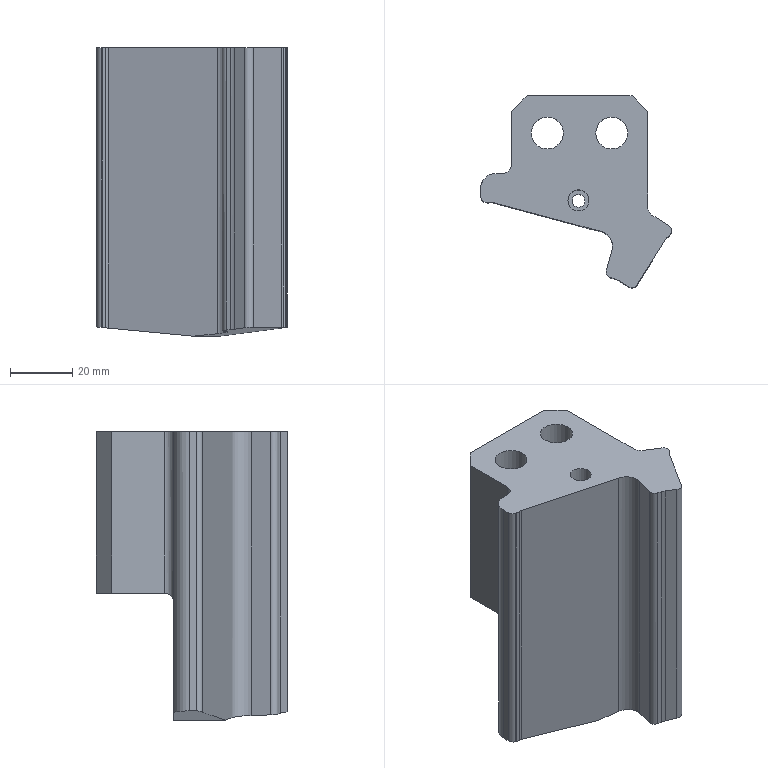Part | NX | features solid 2 | 1 solid | 46 faces | box 61.522 x 61.799 x 92.982 mm | volume 130232 mm3 | plane 22 | cylinder 22 | spline 1 | torus 1 | commonest cylinder face diameters 4 x8 6 x4 10 x4 10.3 x2 17 x2 4.1 x1
STEP:
#1=CARTESIAN_POINT('',(463.121,6.5,50.982));
#2=VERTEX_POINT('',#1);
#3=CARTESIAN_POINT('',(457.971,6.5,50.982));
#4=DIRECTION('',(-0.000000738,0.,-1.));
#5=DIRECTION('',(1.,0.,-0.000000738));
#6=AXIS2_PLACEMENT_3D('',#3,#4,#5);
#7=CIRCLE('',#6,5.15);
#8=EDGE_CURVE('',#2,#2,#7,.F.);
#9=ORIENTED_EDGE('',*,*,#8,.T.);
#10=EDGE_LOOP('',(#9));
#11=FACE_BOUND('',#10,.T.);
#12=CARTESIAN_POINT('',(449.471,6.5,50.982));
#13=VERTEX_POINT('',#12);
#14=CARTESIAN_POINT('',(457.971,6.5,50.982));
#15=DIRECTION('',(0.000000738,0.,1.));
#16=DIRECTION('',(-1.,0.,0.000000738));
#17=AXIS2_PLACEMENT_3D('',#14,#15,#16);
#18=CIRCLE('',#17,8.5);
#19=EDGE_CURVE('',#13,#13,#18,.T.);
#20=ORIENTED_EDGE('',*,*,#19,.F.);
#21=EDGE_LOOP('',(#20));
#22=FACE_BOUND('',#21,.T.);
#23=CARTESIAN_POINT('',(527.356,2.,50.982));
#24=DIRECTION('',(0.000000738,0.,1.));
#25=DIRECTION('',(1.,0.,-0.000000738));
#26=AXIS2_PLACEMENT_3D('',#23,#24,#25);
#27=PLANE('',#26);
#28=ADVANCED_FACE('',(#11,#22),#27,.F.);
#29=ORIENTED_EDGE('',*,*,#19,.T.);
#30=EDGE_LOOP('',(#29));
#31=FACE_BOUND('',#30,.T.);
#32=CARTESIAN_POINT('',(466.471,6.5,26.));
#33=VERTEX_POINT('',#32);
#34=CARTESIAN_POINT('',(457.971,6.5,26.));
#35=DIRECTION('',(0.,0.,1.));
#36=DIRECTION('',(1.,0.,0.));
#37=AXIS2_PLACEMENT_3D('',#34,#35,#36);
#38=CIRCLE('',#37,8.5);
#39=EDGE_CURVE('',#33,#33,#38,.F.);
#40=ORIENTED_EDGE('',*,*,#39,.T.);
#41=EDGE_LOOP('',(#40));
#42=FACE_BOUND('',#41,.T.);
#43=CARTESIAN_POINT('',(457.971,6.5,21.982));
#44=DIRECTION('',(0.000000369,-0.000000231,1.));
#45=DIRECTION('',(-1.,0.,0.000000369));
#46=AXIS2_PLACEMENT_3D('',#43,#44,#45);
#47=CYLINDRICAL_SURFACE('',#46,8.5);
#48=ADVANCED_FACE('',(#31,#42),#47,.F.);
#49=ORIENTED_EDGE('',*,*,#8,.F.);
#50=EDGE_LOOP('',(#49));
#51=FACE_BOUND('',#50,.T.);
#52=CARTESIAN_POINT('',(452.821,6.5,78.));
#53=VERTEX_POINT('',#52);
#54=CARTESIAN_POINT('',(457.971,6.5,78.));
#55=DIRECTION('',(0.,0.,-1.));
#56=DIRECTION('',(-1.,0.,0.));
#57=AXIS2_PLACEMENT_3D('',#54,#55,#56);
#58=CIRCLE('',#57,5.15);
#59=EDGE_CURVE('',#53,#53,#58,.F.);
#60=ORIENTED_EDGE('',*,*,#59,.T.);
#61=EDGE_LOOP('',(#60));
#62=FACE_BOUND('',#61,.T.);
#63=CARTESIAN_POINT('',(457.971,6.5,56.982));
#64=DIRECTION('',(0.000000369,-0.000000231,1.));
#65=DIRECTION('',(-1.,0.,0.000000369));
#66=AXIS2_PLACEMENT_3D('',#63,#64,#65);
#67=CYLINDRICAL_SURFACE('',#66,5.15);
#68=ADVANCED_FACE('',(#51,#62),#67,.F.);
#69=CARTESIAN_POINT('',(447.499,-13.166,-14.982));
#70=VERTEX_POINT('',#69);
#71=CARTESIAN_POINT('',(447.499,-17.238,-14.982));
#72=VERTEX_POINT('',#71);
#73=CARTESIAN_POINT('',(447.26,-15.202,-14.982));
#74=DIRECTION('',(-0.000000369,0.000000231,-1.));
#75=DIRECTION('',(-1.,0.,0.000000369));
#76=AXIS2_PLACEMENT_3D('',#73,#74,#75);
#77=CIRCLE('',#76,2.05);
#78=EDGE_CURVE('',#70,#72,#77,.T.);
#79=ORIENTED_EDGE('',*,*,#78,.F.);
#80=CARTESIAN_POINT('',(447.499,-6.5,-14.982));
#81=VERTEX_POINT('',#80);
#82=CARTESIAN_POINT('',(447.499,-13.942,-14.982));
#83=DIRECTION('',(0.,-1.,-0.000000231));
#84=VECTOR('',#83,1000.);
#85=LINE('',#82,#84);
#86=EDGE_CURVE('',#81,#70,#85,.T.);
#87=ORIENTED_EDGE('',*,*,#86,.F.);
#88=CARTESIAN_POINT('',(448.074,-6.5,-14.982));
#89=VERTEX_POINT('',#88);
#90=CARTESIAN_POINT('',(396.,-6.5,-14.982));
#91=DIRECTION('',(1.,0.,-0.000000369));
#92=VECTOR('',#91,1000.);
#93=LINE('',#90,#92);
#94=EDGE_CURVE('',#81,#89,#93,.T.);
#95=ORIENTED_EDGE('',*,*,#94,.T.);
#96=CARTESIAN_POINT('',(450.724,-7.26,-14.982));
#97=VERTEX_POINT('',#96);
#98=CARTESIAN_POINT('',(448.074,-11.5,-14.982));
#99=DIRECTION('',(0.000000369,-0.000000231,1.));
#100=DIRECTION('',(-1.,0.,0.000000369));
#101=AXIS2_PLACEMENT_3D('',#98,#99,#100);
#102=CIRCLE('',#101,5.);
#103=EDGE_CURVE('',#97,#89,#102,.T.);
#104=ORIENTED_EDGE('',*,*,#103,.F.);
#105=CARTESIAN_POINT('',(454.956,-9.904,-14.982));
#106=VERTEX_POINT('',#105);
#107=CARTESIAN_POINT('',(446.525,-4.636,-14.982));
#108=DIRECTION('',(0.848,-0.5299,-0.000000435));
#109=VECTOR('',#108,1000.);
#110=LINE('',#107,#109);
#111=EDGE_CURVE('',#97,#106,#110,.T.);
#112=ORIENTED_EDGE('',*,*,#111,.T.);
#113=CARTESIAN_POINT('',(447.499,-21.837,-14.982));
#114=VERTEX_POINT('',#113);
#115=CARTESIAN_POINT('',(452.665,-13.57,-14.982));
#116=DIRECTION('',(0.5299,0.848,0.));
#117=VECTOR('',#116,1000.);
#118=LINE('',#115,#117);
#119=EDGE_CURVE('',#114,#106,#118,.T.);
#120=ORIENTED_EDGE('',*,*,#119,.F.);
#121=CARTESIAN_POINT('',(447.499,-13.942,-14.982));
#122=DIRECTION('',(0.,-1.,-0.000000231));
#123=VECTOR('',#122,1000.);
#124=LINE('',#121,#123);
#125=EDGE_CURVE('',#72,#114,#124,.T.);
#126=ORIENTED_EDGE('',*,*,#125,.F.);
#127=EDGE_LOOP('',(#79,#87,#95,#104,#112,#120,#126));
#128=FACE_BOUND('',#127,.T.);
#129=CARTESIAN_POINT('',(393.129,-90.087,-14.982));
#130=DIRECTION('',(-0.000000369,0.000000231,-1.));
#131=DIRECTION('',(-1.,0.,0.000000369));
#132=AXIS2_PLACEMENT_3D('',#129,#130,#131);
#133=PLANE('',#132);
#134=ADVANCED_FACE('',(#128),#133,.T.);
#135=CARTESIAN_POINT('',(442.413,6.5,50.982));
#136=VERTEX_POINT('',#135);
#137=CARTESIAN_POINT('',(437.263,6.5,50.982));
#138=DIRECTION('',(0.,0.,-1.));
#139=DIRECTION('',(1.,0.,0.));
#140=AXIS2_PLACEMENT_3D('',#137,#138,#139);
#141=CIRCLE('',#140,5.15);
#142=EDGE_CURVE('',#136,#136,#141,.F.);
#143=ORIENTED_EDGE('',*,*,#142,.T.);
#144=EDGE_LOOP('',(#143));
#145=FACE_BOUND('',#144,.T.);
#146=CARTESIAN_POINT('',(445.763,6.5,50.982));
#147=VERTEX_POINT('',#146);
#148=CARTESIAN_POINT('',(437.263,6.5,50.982));
#149=DIRECTION('',(0.,0.,-1.));
#150=DIRECTION('',(1.,0.,0.));
#151=AXIS2_PLACEMENT_3D('',#148,#149,#150);
#152=CIRCLE('',#151,8.5);
#153=EDGE_CURVE('',#147,#147,#152,.F.);
#154=ORIENTED_EDGE('',*,*,#153,.F.);
#155=EDGE_LOOP('',(#154));
#156=FACE_BOUND('',#155,.T.);
#157=CARTESIAN_POINT('',(367.879,2.,50.982));
#158=DIRECTION('',(0.,0.,1.));
#159=DIRECTION('',(-1.,0.,0.));
#160=AXIS2_PLACEMENT_3D('',#157,#158,#159);
#161=PLANE('',#160);
#162=ADVANCED_FACE('',(#145,#156),#161,.F.);
#163=CARTESIAN_POINT('',(415.719,-11.5,-11.955));
#164=VERTEX_POINT('',#163);
#165=CARTESIAN_POINT('',(415.719,-11.5,78.));
#166=VERTEX_POINT('',#165);
#167=CARTESIAN_POINT('',(415.719,-11.5,-5.018));
#168=DIRECTION('',(0.000000369,-0.000000231,1.));
#169=VECTOR('',#168,1000.);
#170=LINE('',#167,#169);
#171=EDGE_CURVE('',#164,#166,#170,.T.);
#172=ORIENTED_EDGE('',*,*,#171,.T.);
#173=CARTESIAN_POINT('',(420.719,-6.5,78.));
#174=VERTEX_POINT('',#173);
#175=CARTESIAN_POINT('',(420.719,-11.5,78.));
#176=DIRECTION('',(0.,0.,-1.));
#177=DIRECTION('',(-1.,0.,0.));
#178=AXIS2_PLACEMENT_3D('',#175,#176,#177);
#179=CIRCLE('',#178,5.);
#180=EDGE_CURVE('',#174,#166,#179,.F.);
#181=ORIENTED_EDGE('',*,*,#180,.F.);
#182=CARTESIAN_POINT('',(420.719,-6.5,-12.431));
#183=VERTEX_POINT('',#182);
#184=CARTESIAN_POINT('',(420.719,-6.5,-5.018));
#185=DIRECTION('',(0.000000369,-0.000000231,1.));
#186=VECTOR('',#185,1000.);
#187=LINE('',#184,#186);
#188=EDGE_CURVE('',#183,#174,#187,.T.);
#189=ORIENTED_EDGE('',*,*,#188,.F.);
#190=CARTESIAN_POINT('',(420.719,-11.5,-12.431));
#191=DIRECTION('',(0.09481,-0.00000023,0.9955));
#192=DIRECTION('',(-0.9955,-0.000000022,0.09481));
#193=AXIS2_PLACEMENT_3D('',#190,#191,#192);
#194=ELLIPSE('',#193,5.023,5.);
#195=EDGE_CURVE('',#164,#183,#194,.F.);
#196=ORIENTED_EDGE('',*,*,#195,.F.);
#197=EDGE_LOOP('',(#172,#181,#189,#196));
#198=FACE_BOUND('',#197,.T.);
#199=CARTESIAN_POINT('',(420.719,-11.5,-5.018));
#200=DIRECTION('',(0.000000369,-0.000000231,1.));
#201=DIRECTION('',(1.,0.,-0.000000369));
#202=AXIS2_PLACEMENT_3D('',#199,#200,#201);
#203=CYLINDRICAL_SURFACE('',#202,5.);
#204=ADVANCED_FACE('',(#198),#203,.T.);
#205=CARTESIAN_POINT('',(415.719,-13.767,-11.955));
#206=VERTEX_POINT('',#205);
#207=CARTESIAN_POINT('',(415.719,-13.767,78.));
#208=VERTEX_POINT('',#207);
#209=CARTESIAN_POINT('',(415.719,-13.767,-5.018));
#210=DIRECTION('',(0.000000369,-0.000000231,1.));
#211=VECTOR('',#210,1000.);
#212=LINE('',#209,#211);
#213=EDGE_CURVE('',#206,#208,#212,.T.);
#214=ORIENTED_EDGE('',*,*,#213,.T.);
#215=CARTESIAN_POINT('',(415.719,-0.000000688,78.));
#216=DIRECTION('',(0.,-1.,0.));
#217=VECTOR('',#216,1000.);
#218=LINE('',#215,#217);
#219=EDGE_CURVE('',#166,#208,#218,.T.);
#220=ORIENTED_EDGE('',*,*,#219,.F.);
#221=ORIENTED_EDGE('',*,*,#171,.F.);
#222=CARTESIAN_POINT('',(415.719,-90.087,-11.955));
#223=DIRECTION('',(0.,1.,0.000000231));
#224=VECTOR('',#223,1000.);
#225=LINE('',#222,#224);
#226=EDGE_CURVE('',#206,#164,#225,.T.);
#227=ORIENTED_EDGE('',*,*,#226,.F.);
#228=EDGE_LOOP('',(#214,#220,#221,#227));
#229=FACE_BOUND('',#228,.T.);
#230=CARTESIAN_POINT('',(415.719,-89.912,-5.018));
#231=DIRECTION('',(1.,0.,-0.000000369));
#232=DIRECTION('',(-0.000000369,0.,-1.));
#233=AXIS2_PLACEMENT_3D('',#230,#231,#232);
#234=PLANE('',#233);
#235=ADVANCED_FACE('',(#229),#234,.F.);
#236=CARTESIAN_POINT('',(417.201,-15.698,-12.096));
#237=VERTEX_POINT('',#236);
#238=CARTESIAN_POINT('',(417.201,-15.698,78.));
#239=VERTEX_POINT('',#238);
#240=CARTESIAN_POINT('',(417.201,-15.698,-5.018));
#241=DIRECTION('',(0.000000369,-0.000000231,1.));
#242=VECTOR('',#241,1000.);
#243=LINE('',#240,#242);
#244=EDGE_CURVE('',#237,#239,#243,.T.);
#245=ORIENTED_EDGE('',*,*,#244,.T.);
#246=CARTESIAN_POINT('',(417.719,-13.767,78.));
#247=DIRECTION('',(0.,0.,-1.));
#248=DIRECTION('',(-1.,0.,0.));
#249=AXIS2_PLACEMENT_3D('',#246,#247,#248);
#250=CIRCLE('',#249,2.);
#251=EDGE_CURVE('',#208,#239,#250,.F.);
#252=ORIENTED_EDGE('',*,*,#251,.F.);
#253=ORIENTED_EDGE('',*,*,#213,.F.);
#254=CARTESIAN_POINT('',(417.719,-13.767,-12.145));
#255=DIRECTION('',(0.09481,-0.00000023,0.9955));
#256=DIRECTION('',(-0.9955,-0.000000022,0.09481));
#257=AXIS2_PLACEMENT_3D('',#254,#255,#256);
#258=ELLIPSE('',#257,2.009,2.);
#259=EDGE_CURVE('',#237,#206,#258,.F.);
#260=ORIENTED_EDGE('',*,*,#259,.F.);
#261=EDGE_LOOP('',(#245,#252,#253,#260));
#262=FACE_BOUND('',#261,.T.);
#263=CARTESIAN_POINT('',(417.719,-13.767,-5.018));
#264=DIRECTION('',(0.000000369,-0.000000231,1.));
#265=DIRECTION('',(1.,0.,-0.000000369));
#266=AXIS2_PLACEMENT_3D('',#263,#264,#265);
#267=CYLINDRICAL_SURFACE('',#266,2.);
#268=ADVANCED_FACE('',(#262),#267,.T.);
#269=CARTESIAN_POINT('',(417.626,-15.812,-12.137));
#270=VERTEX_POINT('',#269);
#271=CARTESIAN_POINT('',(417.626,-15.812,78.));
#272=VERTEX_POINT('',#271);
#273=CARTESIAN_POINT('',(417.626,-15.812,-5.018));
#274=DIRECTION('',(0.000000369,-0.000000231,1.));
#275=VECTOR('',#274,1000.);
#276=LINE('',#273,#275);
#277=EDGE_CURVE('',#270,#272,#276,.T.);
#278=ORIENTED_EDGE('',*,*,#277,.T.);
#279=CARTESIAN_POINT('',(291.797,17.903,78.));
#280=DIRECTION('',(0.9659,-0.2588,0.));
#281=VECTOR('',#280,1000.);
#282=LINE('',#279,#281);
#283=EDGE_CURVE('',#239,#272,#282,.T.);
#284=ORIENTED_EDGE('',*,*,#283,.F.);
#285=ORIENTED_EDGE('',*,*,#244,.F.);
#286=CARTESIAN_POINT('',(463.928,-28.219,-16.546));
#287=DIRECTION('',(-0.9619,0.2577,0.09161));
#288=VECTOR('',#287,1000.);
#289=LINE('',#286,#288);
#290=EDGE_CURVE('',#270,#237,#289,.T.);
#291=ORIENTED_EDGE('',*,*,#290,.F.);
#292=EDGE_LOOP('',(#278,#284,#285,#291));
#293=FACE_BOUND('',#292,.T.);
#294=CARTESIAN_POINT('',(402.806,-11.841,-5.018));
#295=DIRECTION('',(0.2588,0.9659,0.000000127));
#296=DIRECTION('',(0.9659,-0.2588,0.));
#297=AXIS2_PLACEMENT_3D('',#294,#295,#296);
#298=PLANE('',#297);
#299=ADVANCED_FACE('',(#293),#298,.F.);
#300=CARTESIAN_POINT('',(418.626,-15.821,-12.232));
#301=VERTEX_POINT('',#300);
#302=CARTESIAN_POINT('',(418.626,-15.821,78.));
#303=VERTEX_POINT('',#302);
#304=CARTESIAN_POINT('',(418.626,-15.821,-5.018));
#305=DIRECTION('',(0.000000369,-0.000000231,1.));
#306=VECTOR('',#305,1000.);
#307=LINE('',#304,#306);
#308=EDGE_CURVE('',#301,#303,#307,.T.);
#309=ORIENTED_EDGE('',*,*,#308,.T.);
#310=CARTESIAN_POINT('',(418.143,-13.88,78.));
#311=DIRECTION('',(0.,0.,-1.));
#312=DIRECTION('',(-1.,0.,0.));
#313=AXIS2_PLACEMENT_3D('',#310,#311,#312);
#314=CIRCLE('',#313,2.);
#315=EDGE_CURVE('',#272,#303,#314,.F.);
#316=ORIENTED_EDGE('',*,*,#315,.F.);
#317=ORIENTED_EDGE('',*,*,#277,.F.);
#318=CARTESIAN_POINT('',(418.143,-13.88,-12.186));
#319=DIRECTION('',(0.09481,-0.00000023,0.9955));
#320=DIRECTION('',(-0.9955,-0.000000022,0.09481));
#321=AXIS2_PLACEMENT_3D('',#318,#319,#320);
#322=ELLIPSE('',#321,2.009,2.);
#323=EDGE_CURVE('',#301,#270,#322,.F.);
#324=ORIENTED_EDGE('',*,*,#323,.F.);
#325=EDGE_LOOP('',(#309,#316,#317,#324));
#326=FACE_BOUND('',#325,.T.);
#327=CARTESIAN_POINT('',(418.143,-13.88,-5.018));
#328=DIRECTION('',(0.000000369,-0.000000231,1.));
#329=DIRECTION('',(1.,0.,-0.000000369));
#330=AXIS2_PLACEMENT_3D('',#327,#328,#329);
#331=CYLINDRICAL_SURFACE('',#330,2.);
#332=ADVANCED_FACE('',(#326),#331,.T.);
#333=CARTESIAN_POINT('',(419.626,-15.83,-12.327));
#334=VERTEX_POINT('',#333);
#335=CARTESIAN_POINT('',(419.626,-15.831,78.));
#336=VERTEX_POINT('',#335);
#337=CARTESIAN_POINT('',(419.626,-15.83,-5.018));
#338=DIRECTION('',(0.000000369,-0.000000231,1.));
#339=VECTOR('',#338,1000.);
#340=LINE('',#337,#339);
#341=EDGE_CURVE('',#334,#336,#340,.T.);
#342=ORIENTED_EDGE('',*,*,#341,.T.);
#343=CARTESIAN_POINT('',(419.108,-17.762,78.));
#344=DIRECTION('',(0.,0.,-1.));
#345=DIRECTION('',(-1.,0.,0.));
#346=AXIS2_PLACEMENT_3D('',#343,#344,#345);
#347=CIRCLE('',#346,2.);
#348=EDGE_CURVE('',#303,#336,#347,.T.);
#349=ORIENTED_EDGE('',*,*,#348,.F.);
#350=ORIENTED_EDGE('',*,*,#308,.F.);
#351=CARTESIAN_POINT('',(419.108,-17.762,-12.278));
#352=DIRECTION('',(0.09481,-0.00000023,0.9955));
#353=DIRECTION('',(-0.9955,-0.000000022,0.09481));
#354=AXIS2_PLACEMENT_3D('',#351,#352,#353);
#355=ELLIPSE('',#354,2.009,2.);
#356=EDGE_CURVE('',#334,#301,#355,.T.);
#357=ORIENTED_EDGE('',*,*,#356,.F.);
#358=EDGE_LOOP('',(#342,#349,#350,#357));
#359=FACE_BOUND('',#358,.T.);
#360=CARTESIAN_POINT('',(419.108,-17.762,-5.018));
#361=DIRECTION('',(0.000000369,-0.000000231,1.));
#362=DIRECTION('',(1.,0.,-0.000000369));
#363=AXIS2_PLACEMENT_3D('',#360,#361,#362);
#364=CYLINDRICAL_SURFACE('',#363,2.);
#365=ADVANCED_FACE('',(#359),#364,.F.);
#366=CARTESIAN_POINT('',(454.551,-25.189,-14.12));
#367=VERTEX_POINT('',#366);
#368=CARTESIAN_POINT('',(447.08,-23.187,-14.942));
#369=VERTEX_POINT('',#368);
#370=CARTESIAN_POINT('',(422.92,-16.713,-17.599));
#371=DIRECTION('',(-0.9605,0.2574,-0.1057));
#372=VECTOR('',#371,1000.);
#373=LINE('',#370,#372);
#374=EDGE_CURVE('',#367,#369,#373,.T.);
#375=ORIENTED_EDGE('',*,*,#374,.F.);
#376=CARTESIAN_POINT('',(454.551,-25.189,78.));
#377=VERTEX_POINT('',#376);
#378=CARTESIAN_POINT('',(454.551,-25.189,-5.018));
#379=DIRECTION('',(0.000000369,-0.000000231,1.));
#380=VECTOR('',#379,1000.);
#381=LINE('',#378,#380);
#382=EDGE_CURVE('',#367,#377,#381,.T.);
#383=ORIENTED_EDGE('',*,*,#382,.T.);
#384=CARTESIAN_POINT('',(291.927,18.386,78.));
#385=DIRECTION('',(0.9659,-0.2588,0.));
#386=VECTOR('',#385,1000.);
#387=LINE('',#384,#386);
#388=EDGE_CURVE('',#336,#377,#387,.T.);
#389=ORIENTED_EDGE('',*,*,#388,.F.);
#390=ORIENTED_EDGE('',*,*,#341,.F.);
#391=CARTESIAN_POINT('',(464.056,-27.736,-16.559));
#392=DIRECTION('',(-0.9619,0.2577,0.09161));
#393=VECTOR('',#392,1000.);
#394=LINE('',#391,#393);
#395=EDGE_CURVE('',#369,#334,#394,.T.);
#396=ORIENTED_EDGE('',*,*,#395,.F.);
#397=EDGE_LOOP('',(#375,#383,#389,#390,#396));
#398=FACE_BOUND('',#397,.T.);
#399=CARTESIAN_POINT('',(419.626,-15.83,-5.018));
#400=DIRECTION('',(0.2588,0.9659,0.000000127));
#401=DIRECTION('',(0.9659,-0.2588,0.));
#402=AXIS2_PLACEMENT_3D('',#399,#400,#401);
#403=PLANE('',#402);
#404=ADVANCED_FACE('',(#398),#403,.F.);
#405=CARTESIAN_POINT('',(458.061,-31.404,-13.423));
#406=VERTEX_POINT('',#405);
#407=CARTESIAN_POINT('',(458.061,-31.404,78.));
#408=VERTEX_POINT('',#407);
#409=CARTESIAN_POINT('',(458.061,-31.404,-5.018));
#410=DIRECTION('',(0.000000369,-0.000000231,1.));
#411=VECTOR('',#410,1000.);
#412=LINE('',#409,#411);
#413=EDGE_CURVE('',#406,#408,#412,.T.);
#414=ORIENTED_EDGE('',*,*,#413,.T.);
#415=CARTESIAN_POINT('',(453.257,-30.018,78.));
#416=DIRECTION('',(0.,0.,-1.));
#417=DIRECTION('',(-1.,0.,0.));
#418=AXIS2_PLACEMENT_3D('',#415,#416,#417);
#419=CIRCLE('',#418,5.);
#420=EDGE_CURVE('',#377,#408,#419,.T.);
#421=ORIENTED_EDGE('',*,*,#420,.F.);
#422=ORIENTED_EDGE('',*,*,#382,.F.);
#423=CARTESIAN_POINT('',(453.257,-30.018,-13.957));
#424=DIRECTION('',(-0.09365,0.05852,0.9939));
#425=DIRECTION('',(0.8429,-0.5267,0.1104));
#426=AXIS2_PLACEMENT_3D('',#423,#424,#425);
#427=ELLIPSE('',#426,5.031,5.);
#428=EDGE_CURVE('',#406,#367,#427,.T.);
#429=ORIENTED_EDGE('',*,*,#428,.F.);
#430=EDGE_LOOP('',(#414,#421,#422,#429));
#431=FACE_BOUND('',#430,.T.);
#432=CARTESIAN_POINT('',(453.257,-30.018,-5.018));
#433=DIRECTION('',(0.000000369,-0.000000231,1.));
#434=DIRECTION('',(1.,0.,-0.000000369));
#435=AXIS2_PLACEMENT_3D('',#432,#433,#434);
#436=CYLINDRICAL_SURFACE('',#435,5.);
#437=ADVANCED_FACE('',(#431),#436,.F.);
#438=CARTESIAN_POINT('',(456.296,-37.575,78.));
#439=VERTEX_POINT('',#438);
#440=CARTESIAN_POINT('',(456.296,-37.575,-13.226));
#441=VERTEX_POINT('',#440);
#442=CARTESIAN_POINT('',(456.296,-37.575,84.982));
#443=DIRECTION('',(0.000000369,-0.000000231,1.));
#444=VECTOR('',#443,1000.);
#445=LINE('',#442,#444);
#446=EDGE_CURVE('',#439,#441,#445,.F.);
#447=ORIENTED_EDGE('',*,*,#446,.F.);
#448=CARTESIAN_POINT('',(458.061,-31.404,78.));
#449=CARTESIAN_POINT('',(457.469,-33.46,78.));
#450=CARTESIAN_POINT('',(456.879,-35.516,78.));
#451=CARTESIAN_POINT('',(456.296,-37.575,78.));
#452=B_SPLINE_CURVE_WITH_KNOTS('',3,(#448,#449,#450,#451),.UNSPECIFIED.,.F.,.F.,(4,4),(0.,0.006418),.UNSPECIFIED.);
#453=EDGE_CURVE('',#408,#439,#452,.T.);
#454=ORIENTED_EDGE('',*,*,#453,.F.);
#455=ORIENTED_EDGE('',*,*,#413,.F.);
#456=CARTESIAN_POINT('',(456.296,-37.575,-13.226));
#457=CARTESIAN_POINT('',(456.879,-35.516,-13.292));
#458=CARTESIAN_POINT('',(457.468,-33.46,-13.358));
#459=CARTESIAN_POINT('',(458.061,-31.404,-13.423));
#460=B_SPLINE_CURVE_WITH_KNOTS('',3,(#456,#457,#458,#459),.UNSPECIFIED.,.F.,.F.,(4,4),(0.,0.006421),.UNSPECIFIED.);
#461=EDGE_CURVE('',#441,#406,#460,.T.);
#462=ORIENTED_EDGE('',*,*,#461,.F.);
#463=EDGE_LOOP('',(#447,#454,#455,#462));
#464=FACE_BOUND('',#463,.T.);
#465=CARTESIAN_POINT('',(458.061,-31.404,-13.972));
#466=CARTESIAN_POINT('',(458.061,-31.404,78.));
#467=CARTESIAN_POINT('',(457.468,-33.46,-13.972));
#468=CARTESIAN_POINT('',(457.469,-33.46,78.));
#469=CARTESIAN_POINT('',(456.879,-35.516,-13.972));
#470=CARTESIAN_POINT('',(456.879,-35.516,78.));
#471=CARTESIAN_POINT('',(456.296,-37.575,-13.972));
#472=CARTESIAN_POINT('',(456.296,-37.575,78.));
#473=B_SPLINE_SURFACE_WITH_KNOTS('',3,1,((#465,#466),(#467,#468),(#469,#470),(#471,#472)),.SURF_OF_LINEAR_EXTRUSION.,.F.,.F.,.F.,(4,4),(2,2),(-0.02584,0.4694),(0.,1.),.PIECEWISE_BEZIER_KNOTS.);
#474=ADVANCED_FACE('',(#464),#473,.T.);
#475=CARTESIAN_POINT('',(457.674,-40.044,-12.951));
#476=VERTEX_POINT('',#475);
#477=CARTESIAN_POINT('',(457.674,-40.044,78.));
#478=VERTEX_POINT('',#477);
#479=CARTESIAN_POINT('',(457.674,-40.044,84.982));
#480=DIRECTION('',(-0.000000369,0.000000231,-1.));
#481=VECTOR('',#480,1000.);
#482=LINE('',#479,#481);
#483=EDGE_CURVE('',#476,#478,#482,.F.);
#484=ORIENTED_EDGE('',*,*,#483,.T.);
#485=CARTESIAN_POINT('',(458.22,-38.12,78.));
#486=DIRECTION('',(0.,0.,-1.));
#487=DIRECTION('',(-1.,0.,0.));
#488=AXIS2_PLACEMENT_3D('',#485,#486,#487);
#489=CIRCLE('',#488,2.);
#490=EDGE_CURVE('',#478,#439,#489,.T.);
#491=ORIENTED_EDGE('',*,*,#490,.T.);
#492=ORIENTED_EDGE('',*,*,#446,.T.);
#493=CARTESIAN_POINT('',(458.22,-38.12,-13.013));
#494=DIRECTION('',(-0.09365,0.05852,0.9939));
#495=DIRECTION('',(0.8429,-0.5267,0.1104));
#496=AXIS2_PLACEMENT_3D('',#493,#494,#495);
#497=ELLIPSE('',#496,2.012,2.);
#498=EDGE_CURVE('',#476,#441,#497,.F.);
#499=ORIENTED_EDGE('',*,*,#498,.F.);
#500=EDGE_LOOP('',(#484,#491,#492,#499));
#501=FACE_BOUND('',#500,.T.);
#502=CARTESIAN_POINT('',(458.22,-38.12,39.982));
#503=DIRECTION('',(0.000000369,-0.000000231,1.));
#504=DIRECTION('',(1.,0.,-0.000000369));
#505=AXIS2_PLACEMENT_3D('',#502,#503,#504);
#506=CYLINDRICAL_SURFACE('',#505,2.);
#507=ADVANCED_FACE('',(#501),#506,.T.);
#508=CARTESIAN_POINT('',(458.771,-40.356,78.));
#509=VERTEX_POINT('',#508);
#510=CARTESIAN_POINT('',(458.771,-40.356,-12.829));
#511=VERTEX_POINT('',#510);
#512=CARTESIAN_POINT('',(458.771,-40.356,-5.018));
#513=DIRECTION('',(0.000000369,-0.000000231,1.));
#514=VECTOR('',#513,1000.);
#515=LINE('',#512,#514);
#516=EDGE_CURVE('',#509,#511,#515,.F.);
#517=ORIENTED_EDGE('',*,*,#516,.F.);
#518=CARTESIAN_POINT('',(289.193,7.734,78.));
#519=DIRECTION('',(-0.9621,0.2728,0.));
#520=VECTOR('',#519,1000.);
#521=LINE('',#518,#520);
#522=EDGE_CURVE('',#509,#478,#521,.T.);
#523=ORIENTED_EDGE('',*,*,#522,.T.);
#524=ORIENTED_EDGE('',*,*,#483,.F.);
#525=CARTESIAN_POINT('',(411.387,-26.918,-18.085));
#526=DIRECTION('',(-0.9566,0.2713,-0.1061));
#527=VECTOR('',#526,1000.);
#528=LINE('',#525,#527);
#529=EDGE_CURVE('',#511,#476,#528,.T.);
#530=ORIENTED_EDGE('',*,*,#529,.F.);
#531=EDGE_LOOP('',(#517,#523,#524,#530));
#532=FACE_BOUND('',#531,.T.);
#533=CARTESIAN_POINT('',(410.762,-26.741,-5.018));
#534=DIRECTION('',(-0.2728,-0.9621,-0.000000121));
#535=DIRECTION('',(-0.9621,0.2728,0.));
#536=AXIS2_PLACEMENT_3D('',#533,#534,#535);
#537=PLANE('',#536);
#538=ADVANCED_FACE('',(#532),#537,.T.);
#539=CARTESIAN_POINT('',(460.056,-40.926,-12.675));
#540=VERTEX_POINT('',#539);
#541=CARTESIAN_POINT('',(460.057,-40.926,78.));
#542=VERTEX_POINT('',#541);
#543=CARTESIAN_POINT('',(460.057,-40.926,84.982));
#544=DIRECTION('',(0.000000369,-0.000000231,1.));
#545=VECTOR('',#544,1000.);
#546=LINE('',#543,#545);
#547=EDGE_CURVE('',#540,#542,#546,.T.);
#548=ORIENTED_EDGE('',*,*,#547,.T.);
#549=CARTESIAN_POINT('',(457.407,-45.166,78.));
#550=DIRECTION('',(0.,0.,-1.));
#551=DIRECTION('',(-1.,0.,0.));
#552=AXIS2_PLACEMENT_3D('',#549,#550,#551);
#553=CIRCLE('',#552,5.);
#554=EDGE_CURVE('',#542,#509,#553,.F.);
#555=ORIENTED_EDGE('',*,*,#554,.T.);
#556=ORIENTED_EDGE('',*,*,#516,.T.);
#557=CARTESIAN_POINT('',(457.407,-45.166,-12.675));
#558=DIRECTION('',(-0.09365,0.05852,0.9939));
#559=DIRECTION('',(-0.8429,0.5267,-0.1104));
#560=AXIS2_PLACEMENT_3D('',#557,#558,#559);
#561=ELLIPSE('',#560,5.031,5.);
#562=EDGE_CURVE('',#540,#511,#561,.T.);
#563=ORIENTED_EDGE('',*,*,#562,.F.);
#564=EDGE_LOOP('',(#548,#555,#556,#563));
#565=FACE_BOUND('',#564,.T.);
#566=CARTESIAN_POINT('',(457.407,-45.166,-5.018));
#567=DIRECTION('',(-0.000000369,0.000000231,-1.));
#568=DIRECTION('',(-1.,0.,0.000000369));
#569=AXIS2_PLACEMENT_3D('',#566,#567,#568);
#570=CYLINDRICAL_SURFACE('',#569,5.);
#571=ADVANCED_FACE('',(#565),#570,.F.);
#572=CARTESIAN_POINT('',(463.368,-42.995,78.));
#573=VERTEX_POINT('',#572);
#574=CARTESIAN_POINT('',(463.368,-42.995,-12.241));
#575=VERTEX_POINT('',#574);
#576=CARTESIAN_POINT('',(463.368,-42.995,-5.018));
#577=DIRECTION('',(-0.000000369,0.000000231,-1.));
#578=VECTOR('',#577,1000.);
#579=LINE('',#576,#578);
#580=EDGE_CURVE('',#573,#575,#579,.T.);
#581=ORIENTED_EDGE('',*,*,#580,.F.);
#582=CARTESIAN_POINT('',(317.205,48.338,78.));
#583=DIRECTION('',(-0.848,0.5299,0.));
#584=VECTOR('',#583,1000.);
#585=LINE('',#582,#584);
#586=EDGE_CURVE('',#573,#542,#585,.T.);
#587=ORIENTED_EDGE('',*,*,#586,.T.);
#588=ORIENTED_EDGE('',*,*,#547,.F.);
#589=CARTESIAN_POINT('',(434.119,-24.718,-16.073));
#590=DIRECTION('',(-0.8429,0.5267,-0.1104));
#591=VECTOR('',#590,1000.);
#592=LINE('',#589,#591);
#593=EDGE_CURVE('',#575,#540,#592,.T.);
#594=ORIENTED_EDGE('',*,*,#593,.F.);
#595=EDGE_LOOP('',(#581,#587,#588,#594));
#596=FACE_BOUND('',#595,.T.);
#597=CARTESIAN_POINT('',(433.735,-24.478,-5.018));
#598=DIRECTION('',(-0.5299,-0.848,0.));
#599=DIRECTION('',(-0.848,0.5299,0.));
#600=AXIS2_PLACEMENT_3D('',#597,#598,#599);
#601=PLANE('',#600);
#602=ADVANCED_FACE('',(#596),#601,.T.);
#603=CARTESIAN_POINT('',(466.124,-42.358,-12.019));
#604=VERTEX_POINT('',#603);
#605=CARTESIAN_POINT('',(466.124,-42.358,78.));
#606=VERTEX_POINT('',#605);
#607=CARTESIAN_POINT('',(466.124,-42.358,84.982));
#608=DIRECTION('',(-0.000000369,0.000000231,-1.));
#609=VECTOR('',#608,1000.);
#610=LINE('',#607,#609);
#611=EDGE_CURVE('',#604,#606,#610,.F.);
#612=ORIENTED_EDGE('',*,*,#611,.T.);
#613=CARTESIAN_POINT('',(464.428,-41.299,78.));
#614=DIRECTION('',(0.,0.,-1.));
#615=DIRECTION('',(-1.,0.,0.));
#616=AXIS2_PLACEMENT_3D('',#613,#614,#615);
#617=CIRCLE('',#616,2.);
#618=EDGE_CURVE('',#606,#573,#617,.T.);
#619=ORIENTED_EDGE('',*,*,#618,.T.);
#620=ORIENTED_EDGE('',*,*,#580,.T.);
#621=CARTESIAN_POINT('',(464.427,-41.299,-12.241));
#622=DIRECTION('',(-0.09365,0.05852,0.9939));
#623=DIRECTION('',(0.8429,-0.5267,0.1104));
#624=AXIS2_PLACEMENT_3D('',#621,#622,#623);
#625=ELLIPSE('',#624,2.012,2.);
#626=EDGE_CURVE('',#604,#575,#625,.F.);
#627=ORIENTED_EDGE('',*,*,#626,.F.);
#628=EDGE_LOOP('',(#612,#619,#620,#627));
#629=FACE_BOUND('',#628,.T.);
#630=CARTESIAN_POINT('',(464.427,-41.299,-5.018));
#631=DIRECTION('',(0.000000369,-0.000000231,1.));
#632=DIRECTION('',(1.,0.,-0.000000369));
#633=AXIS2_PLACEMENT_3D('',#630,#631,#632);
#634=CYLINDRICAL_SURFACE('',#633,2.);
#635=ADVANCED_FACE('',(#629),#634,.T.);
#636=CARTESIAN_POINT('',(475.282,-27.703,-12.019));
#637=VERTEX_POINT('',#636);
#638=CARTESIAN_POINT('',(475.282,-27.703,78.));
#639=VERTEX_POINT('',#638);
#640=CARTESIAN_POINT('',(475.282,-27.703,-5.018));
#641=DIRECTION('',(0.000000369,-0.000000231,1.));
#642=VECTOR('',#641,1000.);
#643=LINE('',#640,#642);
#644=EDGE_CURVE('',#637,#639,#643,.T.);
#645=ORIENTED_EDGE('',*,*,#644,.T.);
#646=CARTESIAN_POINT('',(434.859,-92.392,78.));
#647=DIRECTION('',(0.5299,0.848,0.));
#648=VECTOR('',#647,1000.);
#649=LINE('',#646,#648);
#650=EDGE_CURVE('',#606,#639,#649,.T.);
#651=ORIENTED_EDGE('',*,*,#650,.F.);
#652=ORIENTED_EDGE('',*,*,#611,.F.);
#653=CARTESIAN_POINT('',(424.176,-109.488,-12.019));
#654=DIRECTION('',(-0.5299,-0.848,0.));
#655=VECTOR('',#654,1000.);
#656=LINE('',#653,#655);
#657=EDGE_CURVE('',#637,#604,#656,.T.);
#658=ORIENTED_EDGE('',*,*,#657,.F.);
#659=EDGE_LOOP('',(#645,#651,#652,#658));
#660=FACE_BOUND('',#659,.T.);
#661=CARTESIAN_POINT('',(466.124,-42.358,-5.018));
#662=DIRECTION('',(-0.848,0.5299,0.000000435));
#663=DIRECTION('',(0.5299,0.848,0.));
#664=AXIS2_PLACEMENT_3D('',#661,#662,#663);
#665=PLANE('',#664);
#666=ADVANCED_FACE('',(#660),#665,.F.);
#667=CARTESIAN_POINT('',(476.007,-27.014,-11.991));
#668=VERTEX_POINT('',#667);
#669=CARTESIAN_POINT('',(476.007,-27.014,78.));
#670=VERTEX_POINT('',#669);
#671=CARTESIAN_POINT('',(476.007,-27.014,-5.018));
#672=DIRECTION('',(0.000000369,-0.000000231,1.));
#673=VECTOR('',#672,1000.);
#674=LINE('',#671,#673);
#675=EDGE_CURVE('',#668,#670,#674,.T.);
#676=ORIENTED_EDGE('',*,*,#675,.T.);
#677=CARTESIAN_POINT('',(476.978,-28.763,78.));
#678=DIRECTION('',(0.,0.,-1.));
#679=DIRECTION('',(-1.,0.,0.));
#680=AXIS2_PLACEMENT_3D('',#677,#678,#679);
#681=CIRCLE('',#680,2.);
#682=EDGE_CURVE('',#639,#670,#681,.T.);
#683=ORIENTED_EDGE('',*,*,#682,.F.);
#684=ORIENTED_EDGE('',*,*,#644,.F.);
#685=CARTESIAN_POINT('',(476.978,-28.762,-11.796));
#686=DIRECTION('',(-0.09365,0.05852,0.9939));
#687=DIRECTION('',(0.8429,-0.5267,0.1104));
#688=AXIS2_PLACEMENT_3D('',#685,#686,#687);
#689=ELLIPSE('',#688,2.012,2.);
#690=EDGE_CURVE('',#668,#637,#689,.T.);
#691=ORIENTED_EDGE('',*,*,#690,.F.);
#692=EDGE_LOOP('',(#676,#683,#684,#691));
#693=FACE_BOUND('',#692,.T.);
#694=CARTESIAN_POINT('',(476.978,-28.762,-5.018));
#695=DIRECTION('',(0.000000369,-0.000000231,1.));
#696=DIRECTION('',(1.,0.,-0.000000369));
#697=AXIS2_PLACEMENT_3D('',#694,#695,#696);
#698=CYLINDRICAL_SURFACE('',#697,2.);
#699=ADVANCED_FACE('',(#693),#698,.F.);
#700=CARTESIAN_POINT('',(476.732,-26.325,-11.963));
#701=VERTEX_POINT('',#700);
#702=CARTESIAN_POINT('',(476.732,-26.325,78.));
#703=VERTEX_POINT('',#702);
#704=CARTESIAN_POINT('',(476.732,-26.325,-5.018));
#705=DIRECTION('',(0.000000369,-0.000000231,1.));
#706=VECTOR('',#705,1000.);
#707=LINE('',#704,#706);
#708=EDGE_CURVE('',#701,#703,#707,.T.);
#709=ORIENTED_EDGE('',*,*,#708,.T.);
#710=CARTESIAN_POINT('',(475.036,-25.266,78.));
#711=DIRECTION('',(0.,0.,-1.));
#712=DIRECTION('',(-1.,0.,0.));
#713=AXIS2_PLACEMENT_3D('',#710,#711,#712);
#714=CIRCLE('',#713,2.);
#715=EDGE_CURVE('',#670,#703,#714,.F.);
#716=ORIENTED_EDGE('',*,*,#715,.F.);
#717=ORIENTED_EDGE('',*,*,#675,.F.);
#718=CARTESIAN_POINT('',(475.036,-25.266,-12.185));
#719=DIRECTION('',(-0.09365,0.05852,0.9939));
#720=DIRECTION('',(0.8429,-0.5267,0.1104));
#721=AXIS2_PLACEMENT_3D('',#718,#719,#720);
#722=ELLIPSE('',#721,2.012,2.);
#723=EDGE_CURVE('',#701,#668,#722,.F.);
#724=ORIENTED_EDGE('',*,*,#723,.F.);
#725=EDGE_LOOP('',(#709,#716,#717,#724));
#726=FACE_BOUND('',#725,.T.);
#727=CARTESIAN_POINT('',(475.036,-25.266,-5.018));
#728=DIRECTION('',(0.000000369,-0.000000231,1.));
#729=DIRECTION('',(1.,0.,-0.000000369));
#730=AXIS2_PLACEMENT_3D('',#727,#728,#729);
#731=CYLINDRICAL_SURFACE('',#730,2.);
#732=ADVANCED_FACE('',(#726),#731,.T.);
#733=CARTESIAN_POINT('',(476.936,-25.998,-11.963));
#734=VERTEX_POINT('',#733);
#735=CARTESIAN_POINT('',(476.937,-25.998,78.));
#736=VERTEX_POINT('',#735);
#737=CARTESIAN_POINT('',(476.936,-25.998,-5.018));
#738=DIRECTION('',(0.000000369,-0.000000231,1.));
#739=VECTOR('',#738,1000.);
#740=LINE('',#737,#739);
#741=EDGE_CURVE('',#734,#736,#740,.T.);
#742=ORIENTED_EDGE('',*,*,#741,.T.);
#743=CARTESIAN_POINT('',(435.283,-92.657,78.));
#744=DIRECTION('',(0.5299,0.848,0.));
#745=VECTOR('',#744,1000.);
#746=LINE('',#743,#745);
#747=EDGE_CURVE('',#703,#736,#746,.T.);
#748=ORIENTED_EDGE('',*,*,#747,.F.);
#749=ORIENTED_EDGE('',*,*,#708,.F.);
#750=CARTESIAN_POINT('',(424.6,-109.753,-11.963));
#751=DIRECTION('',(-0.5299,-0.848,0.));
#752=VECTOR('',#751,1000.);
#753=LINE('',#750,#752);
#754=EDGE_CURVE('',#734,#701,#753,.T.);
#755=ORIENTED_EDGE('',*,*,#754,.F.);
#756=EDGE_LOOP('',(#742,#748,#749,#755));
#757=FACE_BOUND('',#756,.T.);
#758=CARTESIAN_POINT('',(474.858,-29.324,-5.018));
#759=DIRECTION('',(-0.848,0.5299,0.000000435));
#760=DIRECTION('',(0.5299,0.848,0.));
#761=AXIS2_PLACEMENT_3D('',#758,#759,#760);
#762=PLANE('',#761);
#763=ADVANCED_FACE('',(#757),#762,.F.);
#764=CARTESIAN_POINT('',(476.3,-23.242,-12.185));
#765=VERTEX_POINT('',#764);
#766=CARTESIAN_POINT('',(476.3,-23.242,78.));
#767=VERTEX_POINT('',#766);
#768=CARTESIAN_POINT('',(476.3,-23.242,-5.018));
#769=DIRECTION('',(0.000000369,-0.000000231,1.));
#770=VECTOR('',#769,1000.);
#771=LINE('',#768,#770);
#772=EDGE_CURVE('',#765,#767,#771,.T.);
#773=ORIENTED_EDGE('',*,*,#772,.T.);
#774=CARTESIAN_POINT('',(475.24,-24.938,78.));
#775=DIRECTION('',(0.,0.,-1.));
#776=DIRECTION('',(-1.,0.,0.));
#777=AXIS2_PLACEMENT_3D('',#774,#775,#776);
#778=CIRCLE('',#777,2.);
#779=EDGE_CURVE('',#736,#767,#778,.F.);
#780=ORIENTED_EDGE('',*,*,#779,.F.);
#781=ORIENTED_EDGE('',*,*,#741,.F.);
#782=CARTESIAN_POINT('',(475.24,-24.938,-12.185));
#783=DIRECTION('',(-0.09365,0.05852,0.9939));
#784=DIRECTION('',(0.8429,-0.5267,0.1104));
#785=AXIS2_PLACEMENT_3D('',#782,#783,#784);
#786=ELLIPSE('',#785,2.012,2.);
#787=EDGE_CURVE('',#765,#734,#786,.F.);
#788=ORIENTED_EDGE('',*,*,#787,.F.);
#789=EDGE_LOOP('',(#773,#780,#781,#788));
#790=FACE_BOUND('',#789,.T.);
#791=CARTESIAN_POINT('',(475.24,-24.938,-5.018));
#792=DIRECTION('',(0.000000369,-0.000000231,1.));
#793=DIRECTION('',(1.,0.,-0.000000369));
#794=AXIS2_PLACEMENT_3D('',#791,#792,#793);
#795=CYLINDRICAL_SURFACE('',#794,2.);
#796=ADVANCED_FACE('',(#790),#795,.T.);
#797=CARTESIAN_POINT('',(470.926,-19.884,78.));
#798=VERTEX_POINT('',#797);
#799=CARTESIAN_POINT('',(470.926,-19.884,23.));
#800=VERTEX_POINT('',#799);
#801=CARTESIAN_POINT('',(470.926,-19.884,-5.018));
#802=DIRECTION('',(-0.000000369,0.000000231,-1.));
#803=VECTOR('',#802,1000.);
#804=LINE('',#801,#803);
#805=EDGE_CURVE('',#798,#800,#804,.T.);
#806=ORIENTED_EDGE('',*,*,#805,.T.);
#807=CARTESIAN_POINT('',(469.516,-17.339,25.544));
#808=VERTEX_POINT('',#807);
#809=CARTESIAN_POINT('',(472.516,-17.339,23.));
#810=DIRECTION('',(-0.5997,0.3747,-0.7071));
#811=DIRECTION('',(0.5997,-0.3747,-0.7071));
#812=AXIS2_PLACEMENT_3D('',#809,#810,#811);
#813=ELLIPSE('',#812,4.243,3.);
#814=EDGE_CURVE('',#800,#808,#813,.T.);
#815=ORIENTED_EDGE('',*,*,#814,.T.);
#816=CARTESIAN_POINT('',(469.516,-17.34,78.));
#817=VERTEX_POINT('',#816);
#818=CARTESIAN_POINT('',(469.516,-17.339,21.982));
#819=DIRECTION('',(0.000000369,-0.000000231,1.));
#820=VECTOR('',#819,1000.);
#821=LINE('',#818,#820);
#822=EDGE_CURVE('',#808,#817,#821,.T.);
#823=ORIENTED_EDGE('',*,*,#822,.T.);
#824=CARTESIAN_POINT('',(472.516,-17.34,78.));
#825=DIRECTION('',(0.,0.,-1.));
#826=DIRECTION('',(-1.,0.,0.));
#827=AXIS2_PLACEMENT_3D('',#824,#825,#826);
#828=CIRCLE('',#827,3.);
#829=EDGE_CURVE('',#817,#798,#828,.F.);
#830=ORIENTED_EDGE('',*,*,#829,.T.);
#831=EDGE_LOOP('',(#806,#815,#823,#830));
#832=FACE_BOUND('',#831,.T.);
#833=CARTESIAN_POINT('',(472.516,-17.339,21.982));
#834=DIRECTION('',(-0.000000369,0.000000231,-1.));
#835=DIRECTION('',(-1.,0.,0.000000369));
#836=AXIS2_PLACEMENT_3D('',#833,#834,#835);
#837=CYLINDRICAL_SURFACE('',#836,3.);
#838=ADVANCED_FACE('',(#832),#837,.F.);
#839=CARTESIAN_POINT('',(450.724,-7.26,23.));
#840=VERTEX_POINT('',#839);
#841=CARTESIAN_POINT('',(450.724,-7.26,-5.018));
#842=DIRECTION('',(0.000000369,-0.000000231,1.));
#843=VECTOR('',#842,1000.);
#844=LINE('',#841,#843);
#845=EDGE_CURVE('',#97,#840,#844,.T.);
#846=ORIENTED_EDGE('',*,*,#845,.T.);
#847=CARTESIAN_POINT('',(446.244,-4.461,23.));
#848=DIRECTION('',(0.848,-0.5299,0.));
#849=VECTOR('',#848,1000.);
#850=LINE('',#847,#849);
#851=EDGE_CURVE('',#840,#800,#850,.T.);
#852=ORIENTED_EDGE('',*,*,#851,.T.);
#853=ORIENTED_EDGE('',*,*,#805,.F.);
#854=CARTESIAN_POINT('',(329.713,68.356,78.));
#855=DIRECTION('',(0.848,-0.5299,0.));
#856=VECTOR('',#855,1000.);
#857=LINE('',#854,#856);
#858=EDGE_CURVE('',#798,#767,#857,.T.);
#859=ORIENTED_EDGE('',*,*,#858,.T.);
#860=ORIENTED_EDGE('',*,*,#772,.F.);
#861=CARTESIAN_POINT('',(446.628,-4.7,-16.073));
#862=DIRECTION('',(0.8429,-0.5267,0.1104));
#863=VECTOR('',#862,1000.);
#864=LINE('',#861,#863);
#865=EDGE_CURVE('',#106,#765,#864,.T.);
#866=ORIENTED_EDGE('',*,*,#865,.F.);
#867=ORIENTED_EDGE('',*,*,#111,.F.);
#868=EDGE_LOOP('',(#846,#852,#853,#859,#860,#866,#867));
#869=FACE_BOUND('',#868,.T.);
#870=CARTESIAN_POINT('',(446.244,-4.461,-5.018));
#871=DIRECTION('',(0.5299,0.848,0.));
#872=DIRECTION('',(0.848,-0.5299,0.));
#873=AXIS2_PLACEMENT_3D('',#870,#871,#872);
#874=PLANE('',#873);
#875=ADVANCED_FACE('',(#869),#874,.T.);
#876=CARTESIAN_POINT('',(448.074,-6.5,23.));
#877=VERTEX_POINT('',#876);
#878=CARTESIAN_POINT('',(448.074,-6.5,-5.018));
#879=DIRECTION('',(0.000000369,-0.000000231,1.));
#880=VECTOR('',#879,1000.);
#881=LINE('',#878,#880);
#882=EDGE_CURVE('',#89,#877,#881,.T.);
#883=ORIENTED_EDGE('',*,*,#882,.T.);
#884=CARTESIAN_POINT('',(448.074,-11.5,23.));
#885=DIRECTION('',(0.,0.,1.));
#886=DIRECTION('',(1.,0.,0.));
#887=AXIS2_PLACEMENT_3D('',#884,#885,#886);
#888=CIRCLE('',#887,5.);
#889=EDGE_CURVE('',#877,#840,#888,.F.);
#890=ORIENTED_EDGE('',*,*,#889,.T.);
#891=ORIENTED_EDGE('',*,*,#845,.F.);
#892=ORIENTED_EDGE('',*,*,#103,.T.);
#893=EDGE_LOOP('',(#883,#890,#891,#892));
#894=FACE_BOUND('',#893,.T.);
#895=CARTESIAN_POINT('',(448.074,-11.5,-5.018));
#896=DIRECTION('',(0.000000369,-0.000000231,1.));
#897=DIRECTION('',(1.,0.,-0.000000369));
#898=AXIS2_PLACEMENT_3D('',#895,#896,#897);
#899=CYLINDRICAL_SURFACE('',#898,5.);
#900=ADVANCED_FACE('',(#894),#899,.T.);
#901=CARTESIAN_POINT('',(422.719,-6.5,23.));
#902=VERTEX_POINT('',#901);
#903=CARTESIAN_POINT('',(422.719,-6.5,78.));
#904=VERTEX_POINT('',#903);
#905=CARTESIAN_POINT('',(422.719,-6.5,-5.018));
#906=DIRECTION('',(0.000000369,-0.000000231,1.));
#907=VECTOR('',#906,1000.);
#908=LINE('',#905,#907);
#909=EDGE_CURVE('',#902,#904,#908,.T.);
#910=ORIENTED_EDGE('',*,*,#909,.F.);
#911=CARTESIAN_POINT('',(396.,-6.5,23.));
#912=DIRECTION('',(1.,0.,0.));
#913=VECTOR('',#912,1000.);
#914=LINE('',#911,#913);
#915=EDGE_CURVE('',#902,#877,#914,.T.);
#916=ORIENTED_EDGE('',*,*,#915,.T.);
#917=ORIENTED_EDGE('',*,*,#882,.F.);
#918=ORIENTED_EDGE('',*,*,#94,.F.);
#919=CARTESIAN_POINT('',(396.182,-6.5,-10.094));
#920=DIRECTION('',(0.9955,0.000000022,-0.09481));
#921=VECTOR('',#920,1000.);
#922=LINE('',#919,#921);
#923=EDGE_CURVE('',#183,#81,#922,.T.);
#924=ORIENTED_EDGE('',*,*,#923,.F.);
#925=ORIENTED_EDGE('',*,*,#188,.T.);
#926=CARTESIAN_POINT('',(287.,-6.5,78.));
#927=DIRECTION('',(1.,0.,0.));
#928=VECTOR('',#927,1000.);
#929=LINE('',#926,#928);
#930=EDGE_CURVE('',#174,#904,#929,.T.);
#931=ORIENTED_EDGE('',*,*,#930,.T.);
#932=EDGE_LOOP('',(#910,#916,#917,#918,#924,#925,#931));
#933=FACE_BOUND('',#932,.T.);
#934=CARTESIAN_POINT('',(396.,-6.5,-5.018));
#935=DIRECTION('',(0.,1.,0.000000231));
#936=DIRECTION('',(0.,0.000000231,-1.));
#937=AXIS2_PLACEMENT_3D('',#934,#935,#936);
#938=PLANE('',#937);
#939=ADVANCED_FACE('',(#933),#938,.T.);
#940=CARTESIAN_POINT('',(425.719,-3.5,78.));
#941=VERTEX_POINT('',#940);
#942=CARTESIAN_POINT('',(425.719,-3.5,26.));
#943=VERTEX_POINT('',#942);
#944=CARTESIAN_POINT('',(425.719,-3.5,-5.018));
#945=DIRECTION('',(0.000000369,-0.000000231,1.));
#946=VECTOR('',#945,1000.);
#947=LINE('',#944,#946);
#948=EDGE_CURVE('',#941,#943,#947,.F.);
#949=ORIENTED_EDGE('',*,*,#948,.T.);
#950=CARTESIAN_POINT('',(422.719,-3.5,23.));
#951=DIRECTION('',(-0.7071,-0.000000163,0.7071));
#952=DIRECTION('',(0.7071,-0.000000163,0.7071));
#953=AXIS2_PLACEMENT_3D('',#950,#951,#952);
#954=ELLIPSE('',#953,4.243,3.);
#955=EDGE_CURVE('',#943,#902,#954,.F.);
#956=ORIENTED_EDGE('',*,*,#955,.T.);
#957=ORIENTED_EDGE('',*,*,#909,.T.);
#958=CARTESIAN_POINT('',(422.719,-3.5,78.));
#959=DIRECTION('',(0.,0.,-1.));
#960=DIRECTION('',(-1.,0.,0.));
#961=AXIS2_PLACEMENT_3D('',#958,#959,#960);
#962=CIRCLE('',#961,3.);
#963=EDGE_CURVE('',#904,#941,#962,.F.);
#964=ORIENTED_EDGE('',*,*,#963,.T.);
#965=EDGE_LOOP('',(#949,#956,#957,#964));
#966=FACE_BOUND('',#965,.T.);
#967=CARTESIAN_POINT('',(422.719,-3.5,-5.018));
#968=DIRECTION('',(0.000000369,-0.000000231,1.));
#969=DIRECTION('',(1.,0.,-0.000000369));
#970=AXIS2_PLACEMENT_3D('',#967,#968,#969);
#971=CYLINDRICAL_SURFACE('',#970,3.);
#972=ADVANCED_FACE('',(#966),#971,.F.);
#973=CARTESIAN_POINT('',(425.719,13.5,26.));
#974=VERTEX_POINT('',#973);
#975=CARTESIAN_POINT('',(425.719,-6.5,26.));
#976=DIRECTION('',(0.,-1.,0.));
#977=VECTOR('',#976,1000.);
#978=LINE('',#975,#977);
#979=EDGE_CURVE('',#974,#943,#978,.T.);
#980=ORIENTED_EDGE('',*,*,#979,.T.);
#981=ORIENTED_EDGE('',*,*,#948,.F.);
#982=CARTESIAN_POINT('',(425.719,13.5,78.));
#983=VERTEX_POINT('',#982);
#984=CARTESIAN_POINT('',(425.719,-0.000000688,78.));
#985=DIRECTION('',(0.,-1.,0.));
#986=VECTOR('',#985,1000.);
#987=LINE('',#984,#986);
#988=EDGE_CURVE('',#983,#941,#987,.T.);
#989=ORIENTED_EDGE('',*,*,#988,.F.);
#990=CARTESIAN_POINT('',(425.719,13.5,84.982));
#991=DIRECTION('',(0.000000369,-0.000000231,1.));
#992=VECTOR('',#991,1000.);
#993=LINE('',#990,#992);
#994=EDGE_CURVE('',#974,#983,#993,.T.);
#995=ORIENTED_EDGE('',*,*,#994,.F.);
#996=EDGE_LOOP('',(#980,#981,#989,#995));
#997=FACE_BOUND('',#996,.T.);
#998=CARTESIAN_POINT('',(425.719,-6.5,-5.018));
#999=DIRECTION('',(1.,0.,-0.000000369));
#1000=DIRECTION('',(0.000000369,-0.000000231,1.));
#1001=AXIS2_PLACEMENT_3D('',#998,#999,#1000);
#1002=PLANE('',#1001);
#1003=ADVANCED_FACE('',(#997),#1002,.F.);
#1004=CARTESIAN_POINT('',(430.719,18.5,26.));
#1005=VERTEX_POINT('',#1004);
#1006=CARTESIAN_POINT('',(318.762,-93.456,26.));
#1007=DIRECTION('',(-0.7071,-0.7071,0.));
#1008=VECTOR('',#1007,1000.);
#1009=LINE('',#1006,#1008);
#1010=EDGE_CURVE('',#1005,#974,#1009,.T.);
#1011=ORIENTED_EDGE('',*,*,#1010,.T.);
#1012=ORIENTED_EDGE('',*,*,#994,.T.);
#1013=CARTESIAN_POINT('',(430.719,18.5,78.));
#1014=VERTEX_POINT('',#1013);
#1015=CARTESIAN_POINT('',(349.609,-62.609,78.));
#1016=DIRECTION('',(0.7071,0.7071,0.));
#1017=VECTOR('',#1016,1000.);
#1018=LINE('',#1015,#1017);
#1019=EDGE_CURVE('',#983,#1014,#1018,.T.);
#1020=ORIENTED_EDGE('',*,*,#1019,.T.);
#1021=CARTESIAN_POINT('',(430.719,18.5,21.982));
#1022=DIRECTION('',(-0.000000369,0.000000231,-1.));
#1023=VECTOR('',#1022,1000.);
#1024=LINE('',#1021,#1023);
#1025=EDGE_CURVE('',#1014,#1005,#1024,.T.);
#1026=ORIENTED_EDGE('',*,*,#1025,.T.);
#1027=EDGE_LOOP('',(#1011,#1012,#1020,#1026));
#1028=FACE_BOUND('',#1027,.T.);
#1029=CARTESIAN_POINT('',(425.719,13.5,-5.018));
#1030=DIRECTION('',(-0.7071,0.7071,0.000000424));
#1031=DIRECTION('',(-0.000000369,0.000000231,-1.));
#1032=AXIS2_PLACEMENT_3D('',#1029,#1030,#1031);
#1033=PLANE('',#1032);
#1034=ADVANCED_FACE('',(#1028),#1033,.T.);
#1035=CARTESIAN_POINT('',(464.516,18.5,26.));
#1036=VERTEX_POINT('',#1035);
#1037=CARTESIAN_POINT('',(396.,18.5,26.));
#1038=DIRECTION('',(1.,0.,0.));
#1039=VECTOR('',#1038,1000.);
#1040=LINE('',#1037,#1039);
#1041=EDGE_CURVE('',#1005,#1036,#1040,.T.);
#1042=ORIENTED_EDGE('',*,*,#1041,.F.);
#1043=ORIENTED_EDGE('',*,*,#1025,.F.);
#1044=CARTESIAN_POINT('',(464.516,18.5,78.));
#1045=VERTEX_POINT('',#1044);
#1046=CARTESIAN_POINT('',(287.,18.5,78.));
#1047=DIRECTION('',(1.,0.,0.));
#1048=VECTOR('',#1047,1000.);
#1049=LINE('',#1046,#1048);
#1050=EDGE_CURVE('',#1014,#1045,#1049,.T.);
#1051=ORIENTED_EDGE('',*,*,#1050,.T.);
#1052=CARTESIAN_POINT('',(464.516,18.5,84.982));
#1053=DIRECTION('',(0.000000369,-0.000000231,1.));
#1054=VECTOR('',#1053,1000.);
#1055=LINE('',#1052,#1054);
#1056=EDGE_CURVE('',#1036,#1045,#1055,.T.);
#1057=ORIENTED_EDGE('',*,*,#1056,.F.);
#1058=EDGE_LOOP('',(#1042,#1043,#1051,#1057));
#1059=FACE_BOUND('',#1058,.T.);
#1060=CARTESIAN_POINT('',(396.,18.5,-5.018));
#1061=DIRECTION('',(0.,1.,0.000000231));
#1062=DIRECTION('',(0.,0.000000231,-1.));
#1063=AXIS2_PLACEMENT_3D('',#1060,#1061,#1062);
#1064=PLANE('',#1063);
#1065=ADVANCED_FACE('',(#1059),#1064,.T.);
#1066=CARTESIAN_POINT('',(469.516,13.5,26.));
#1067=VERTEX_POINT('',#1066);
#1068=CARTESIAN_POINT('',(380.145,102.871,26.));
#1069=DIRECTION('',(0.7071,-0.7071,0.));
#1070=VECTOR('',#1069,1000.);
#1071=LINE('',#1068,#1070);
#1072=EDGE_CURVE('',#1067,#1036,#1071,.F.);
#1073=ORIENTED_EDGE('',*,*,#1072,.T.);
#1074=ORIENTED_EDGE('',*,*,#1056,.T.);
#1075=CARTESIAN_POINT('',(469.516,13.5,78.));
#1076=VERTEX_POINT('',#1075);
#1077=CARTESIAN_POINT('',(385.008,98.008,78.));
#1078=DIRECTION('',(-0.7071,0.7071,0.));
#1079=VECTOR('',#1078,1000.);
#1080=LINE('',#1077,#1079);
#1081=EDGE_CURVE('',#1045,#1076,#1080,.F.);
#1082=ORIENTED_EDGE('',*,*,#1081,.T.);
#1083=CARTESIAN_POINT('',(469.516,13.5,21.982));
#1084=DIRECTION('',(0.000000369,-0.000000231,1.));
#1085=VECTOR('',#1084,1000.);
#1086=LINE('',#1083,#1085);
#1087=EDGE_CURVE('',#1076,#1067,#1086,.F.);
#1088=ORIENTED_EDGE('',*,*,#1087,.T.);
#1089=EDGE_LOOP('',(#1073,#1074,#1082,#1088));
#1090=FACE_BOUND('',#1089,.T.);
#1091=CARTESIAN_POINT('',(464.516,18.5,-5.018));
#1092=DIRECTION('',(-0.7071,-0.7071,0.000000098));
#1093=DIRECTION('',(0.000000369,-0.000000231,1.));
#1094=AXIS2_PLACEMENT_3D('',#1091,#1092,#1093);
#1095=PLANE('',#1094);
#1096=ADVANCED_FACE('',(#1090),#1095,.F.);
#1097=CARTESIAN_POINT('',(469.516,-119.002,78.));
#1098=DIRECTION('',(0.,1.,0.));
#1099=VECTOR('',#1098,1000.);
#1100=LINE('',#1097,#1099);
#1101=EDGE_CURVE('',#1076,#817,#1100,.F.);
#1102=ORIENTED_EDGE('',*,*,#1101,.T.);
#1103=ORIENTED_EDGE('',*,*,#822,.F.);
#1104=CARTESIAN_POINT('',(469.516,-15.465,26.));
#1105=VERTEX_POINT('',#1104);
#1106=CARTESIAN_POINT('',(469.516,-15.465,23.));
#1107=DIRECTION('',(1.,0.,-0.000000369));
#1108=DIRECTION('',(0.,-1.,0.000000591));
#1109=AXIS2_PLACEMENT_3D('',#1106,#1107,#1108);
#1110=ELLIPSE('',#1109,3.538,3.);
#1111=EDGE_CURVE('',#808,#1105,#1110,.F.);
#1112=ORIENTED_EDGE('',*,*,#1111,.T.);
#1113=CARTESIAN_POINT('',(469.516,-25.984,26.));
#1114=DIRECTION('',(0.,1.,0.));
#1115=VECTOR('',#1114,1000.);
#1116=LINE('',#1113,#1115);
#1117=EDGE_CURVE('',#1067,#1105,#1116,.F.);
#1118=ORIENTED_EDGE('',*,*,#1117,.F.);
#1119=ORIENTED_EDGE('',*,*,#1087,.F.);
#1120=EDGE_LOOP('',(#1102,#1103,#1112,#1118,#1119));
#1121=FACE_BOUND('',#1120,.T.);
#1122=CARTESIAN_POINT('',(469.516,-119.002,21.982));
#1123=DIRECTION('',(1.,0.,-0.000000369));
#1124=DIRECTION('',(-0.000000369,0.,-1.));
#1125=AXIS2_PLACEMENT_3D('',#1122,#1123,#1124);
#1126=PLANE('',#1125);
#1127=ADVANCED_FACE('',(#1121),#1126,.T.);
#1128=ORIENTED_EDGE('',*,*,#153,.T.);
#1129=EDGE_LOOP('',(#1128));
#1130=FACE_BOUND('',#1129,.T.);
#1131=CARTESIAN_POINT('',(445.763,6.5,26.));
#1132=VERTEX_POINT('',#1131);
#1133=CARTESIAN_POINT('',(437.263,6.5,26.));
#1134=DIRECTION('',(0.,0.,1.));
#1135=DIRECTION('',(1.,0.,0.));
#1136=AXIS2_PLACEMENT_3D('',#1133,#1134,#1135);
#1137=CIRCLE('',#1136,8.5);
#1138=EDGE_CURVE('',#1132,#1132,#1137,.F.);
#1139=ORIENTED_EDGE('',*,*,#1138,.T.);
#1140=EDGE_LOOP('',(#1139));
#1141=FACE_BOUND('',#1140,.T.);
#1142=CARTESIAN_POINT('',(437.263,6.5,21.982));
#1143=DIRECTION('',(0.000000369,-0.000000231,1.));
#1144=DIRECTION('',(1.,0.,-0.000000369));
#1145=AXIS2_PLACEMENT_3D('',#1142,#1143,#1144);
#1146=CYLINDRICAL_SURFACE('',#1145,8.5);
#1147=ADVANCED_FACE('',(#1130,#1141),#1146,.F.);
#1148=ORIENTED_EDGE('',*,*,#39,.F.);
#1149=EDGE_LOOP('',(#1148));
#1150=FACE_BOUND('',#1149,.T.);
#1151=ORIENTED_EDGE('',*,*,#1138,.F.);
#1152=EDGE_LOOP('',(#1151));
#1153=FACE_BOUND('',#1152,.T.);
#1154=CARTESIAN_POINT('',(452.313,-4.716,26.));
#1155=VERTEX_POINT('',#1154);
#1156=CARTESIAN_POINT('',(448.074,-3.5,26.));
#1157=VERTEX_POINT('',#1156);
#1158=CARTESIAN_POINT('',(448.074,-11.5,26.));
#1159=DIRECTION('',(0.,0.,1.));
#1160=DIRECTION('',(1.,0.,0.));
#1161=AXIS2_PLACEMENT_3D('',#1158,#1159,#1160);
#1162=CIRCLE('',#1161,8.);
#1163=EDGE_CURVE('',#1155,#1157,#1162,.T.);
#1164=ORIENTED_EDGE('',*,*,#1163,.T.);
#1165=CARTESIAN_POINT('',(251.29,-3.5,26.));
#1166=DIRECTION('',(1.,0.,0.));
#1167=VECTOR('',#1166,1000.);
#1168=LINE('',#1165,#1167);
#1169=EDGE_CURVE('',#1157,#943,#1168,.F.);
#1170=ORIENTED_EDGE('',*,*,#1169,.T.);
#1171=ORIENTED_EDGE('',*,*,#979,.F.);
#1172=ORIENTED_EDGE('',*,*,#1010,.F.);
#1173=ORIENTED_EDGE('',*,*,#1041,.T.);
#1174=ORIENTED_EDGE('',*,*,#1072,.F.);
#1175=ORIENTED_EDGE('',*,*,#1117,.T.);
#1176=CARTESIAN_POINT('',(317.298,79.651,26.));
#1177=DIRECTION('',(0.848,-0.5299,0.));
#1178=VECTOR('',#1177,1000.);
#1179=LINE('',#1176,#1178);
#1180=EDGE_CURVE('',#1105,#1155,#1179,.F.);
#1181=ORIENTED_EDGE('',*,*,#1180,.T.);
#1182=EDGE_LOOP('',(#1164,#1170,#1171,#1172,#1173,#1174,#1175,#1181));
#1183=FACE_BOUND('',#1182,.T.);
#1184=CARTESIAN_POINT('',(251.29,-25.984,26.));
#1185=DIRECTION('',(0.,0.,1.));
#1186=DIRECTION('',(1.,0.,0.));
#1187=AXIS2_PLACEMENT_3D('',#1184,#1185,#1186);
#1188=PLANE('',#1187);
#1189=ADVANCED_FACE('',(#1150,#1153,#1183),#1188,.F.);
#1190=ORIENTED_EDGE('',*,*,#142,.F.);
#1191=EDGE_LOOP('',(#1190));
#1192=FACE_BOUND('',#1191,.T.);
#1193=CARTESIAN_POINT('',(432.113,6.5,78.));
#1194=VERTEX_POINT('',#1193);
#1195=CARTESIAN_POINT('',(437.263,6.5,78.));
#1196=DIRECTION('',(0.,0.,-1.));
#1197=DIRECTION('',(-1.,0.,0.));
#1198=AXIS2_PLACEMENT_3D('',#1195,#1196,#1197);
#1199=CIRCLE('',#1198,5.15);
#1200=EDGE_CURVE('',#1194,#1194,#1199,.T.);
#1201=ORIENTED_EDGE('',*,*,#1200,.F.);
#1202=EDGE_LOOP('',(#1201));
#1203=FACE_BOUND('',#1202,.T.);
#1204=CARTESIAN_POINT('',(437.263,6.5,56.982));
#1205=DIRECTION('',(0.000000369,-0.000000231,1.));
#1206=DIRECTION('',(1.,0.,-0.000000369));
#1207=AXIS2_PLACEMENT_3D('',#1204,#1205,#1206);
#1208=CYLINDRICAL_SURFACE('',#1207,5.15);
#1209=ADVANCED_FACE('',(#1192,#1203),#1208,.F.);
#1210=CARTESIAN_POINT('',(443.86,-15.202,78.));
#1211=VERTEX_POINT('',#1210);
#1212=CARTESIAN_POINT('',(447.26,-15.202,78.));
#1213=DIRECTION('',(0.,0.,-1.));
#1214=DIRECTION('',(-1.,0.,0.));
#1215=AXIS2_PLACEMENT_3D('',#1212,#1213,#1214);
#1216=CIRCLE('',#1215,3.4);
#1217=EDGE_CURVE('',#1211,#1211,#1216,.T.);
#1218=ORIENTED_EDGE('',*,*,#1217,.T.);
#1219=EDGE_LOOP('',(#1218));
#1220=FACE_BOUND('',#1219,.T.);
#1221=ORIENTED_EDGE('',*,*,#59,.F.);
#1222=EDGE_LOOP('',(#1221));
#1223=FACE_BOUND('',#1222,.T.);
#1224=ORIENTED_EDGE('',*,*,#1200,.T.);
#1225=EDGE_LOOP('',(#1224));
#1226=FACE_BOUND('',#1225,.T.);
#1227=ORIENTED_EDGE('',*,*,#1050,.F.);
#1228=ORIENTED_EDGE('',*,*,#1019,.F.);
#1229=ORIENTED_EDGE('',*,*,#988,.T.);
#1230=ORIENTED_EDGE('',*,*,#963,.F.);
#1231=ORIENTED_EDGE('',*,*,#930,.F.);
#1232=ORIENTED_EDGE('',*,*,#180,.T.);
#1233=ORIENTED_EDGE('',*,*,#219,.T.);
#1234=ORIENTED_EDGE('',*,*,#251,.T.);
#1235=ORIENTED_EDGE('',*,*,#283,.T.);
#1236=ORIENTED_EDGE('',*,*,#315,.T.);
#1237=ORIENTED_EDGE('',*,*,#348,.T.);
#1238=ORIENTED_EDGE('',*,*,#388,.T.);
#1239=ORIENTED_EDGE('',*,*,#420,.T.);
#1240=ORIENTED_EDGE('',*,*,#453,.T.);
#1241=ORIENTED_EDGE('',*,*,#490,.F.);
#1242=ORIENTED_EDGE('',*,*,#522,.F.);
#1243=ORIENTED_EDGE('',*,*,#554,.F.);
#1244=ORIENTED_EDGE('',*,*,#586,.F.);
#1245=ORIENTED_EDGE('',*,*,#618,.F.);
#1246=ORIENTED_EDGE('',*,*,#650,.T.);
#1247=ORIENTED_EDGE('',*,*,#682,.T.);
#1248=ORIENTED_EDGE('',*,*,#715,.T.);
#1249=ORIENTED_EDGE('',*,*,#747,.T.);
#1250=ORIENTED_EDGE('',*,*,#779,.T.);
#1251=ORIENTED_EDGE('',*,*,#858,.F.);
#1252=ORIENTED_EDGE('',*,*,#829,.F.);
#1253=ORIENTED_EDGE('',*,*,#1101,.F.);
#1254=ORIENTED_EDGE('',*,*,#1081,.F.);
#1255=EDGE_LOOP('',(#1227,#1228,#1229,#1230,#1231,#1232,#1233,#1234,#1235,#1236,#1237,#1238,#1239,#1240,#1241,#1242,#1243,#1244,#1245,#1246,#1247,#1248,#1249,#1250,#1251,#1252,#1253,#1254));
#1256=FACE_BOUND('',#1255,.T.);
#1257=CARTESIAN_POINT('',(287.,-0.000000688,78.));
#1258=DIRECTION('',(0.,0.,-1.));
#1259=DIRECTION('',(-1.,0.,0.));
#1260=AXIS2_PLACEMENT_3D('',#1257,#1258,#1259);
#1261=PLANE('',#1260);
#1262=ADVANCED_FACE('',(#1220,#1223,#1226,#1256),#1261,.F.);
#1263=ORIENTED_EDGE('',*,*,#119,.T.);
#1264=ORIENTED_EDGE('',*,*,#865,.T.);
#1265=ORIENTED_EDGE('',*,*,#787,.T.);
#1266=ORIENTED_EDGE('',*,*,#754,.T.);
#1267=ORIENTED_EDGE('',*,*,#723,.T.);
#1268=ORIENTED_EDGE('',*,*,#690,.T.);
#1269=ORIENTED_EDGE('',*,*,#657,.T.);
#1270=ORIENTED_EDGE('',*,*,#626,.T.);
#1271=ORIENTED_EDGE('',*,*,#593,.T.);
#1272=ORIENTED_EDGE('',*,*,#562,.T.);
#1273=ORIENTED_EDGE('',*,*,#529,.T.);
#1274=ORIENTED_EDGE('',*,*,#498,.T.);
#1275=ORIENTED_EDGE('',*,*,#461,.T.);
#1276=ORIENTED_EDGE('',*,*,#428,.T.);
#1277=ORIENTED_EDGE('',*,*,#374,.T.);
#1278=CARTESIAN_POINT('',(422.638,-101.836,-12.614));
#1279=DIRECTION('',(-0.2966,-0.9546,0.02825));
#1280=VECTOR('',#1279,1000.);
#1281=LINE('',#1278,#1280);
#1282=EDGE_CURVE('',#114,#369,#1281,.T.);
#1283=ORIENTED_EDGE('',*,*,#1282,.F.);
#1284=EDGE_LOOP('',(#1263,#1264,#1265,#1266,#1267,#1268,#1269,#1270,#1271,#1272,#1273,#1274,#1275,#1276,#1277,#1283));
#1285=FACE_BOUND('',#1284,.T.);
#1286=CARTESIAN_POINT('',(401.56,-95.356,-14.982));
#1287=DIRECTION('',(0.09365,-0.05852,-0.9939));
#1288=DIRECTION('',(-0.5299,-0.848,0.));
#1289=AXIS2_PLACEMENT_3D('',#1286,#1287,#1288);
#1290=PLANE('',#1289);
#1291=ADVANCED_FACE('',(#1285),#1290,.T.);
#1292=CARTESIAN_POINT('',(447.26,-15.202,-14.959));
#1293=DIRECTION('',(-0.09481,0.00000023,-0.9955));
#1294=DIRECTION('',(-0.9955,0.000002411,0.09481));
#1295=AXIS2_PLACEMENT_3D('',#1292,#1293,#1294);
#1296=ELLIPSE('',#1295,2.059,2.05);
#1297=EDGE_CURVE('',#72,#70,#1296,.T.);
#1298=ORIENTED_EDGE('',*,*,#1297,.F.);
#1299=ORIENTED_EDGE('',*,*,#125,.T.);
#1300=ORIENTED_EDGE('',*,*,#1282,.T.);
#1301=ORIENTED_EDGE('',*,*,#395,.T.);
#1302=ORIENTED_EDGE('',*,*,#356,.T.);
#1303=ORIENTED_EDGE('',*,*,#323,.T.);
#1304=ORIENTED_EDGE('',*,*,#290,.T.);
#1305=ORIENTED_EDGE('',*,*,#259,.T.);
#1306=ORIENTED_EDGE('',*,*,#226,.T.);
#1307=ORIENTED_EDGE('',*,*,#195,.T.);
#1308=ORIENTED_EDGE('',*,*,#923,.T.);
#1309=ORIENTED_EDGE('',*,*,#86,.T.);
#1310=EDGE_LOOP('',(#1298,#1299,#1300,#1301,#1302,#1303,#1304,#1305,#1306,#1307,#1308,#1309));
#1311=FACE_BOUND('',#1310,.T.);
#1312=CARTESIAN_POINT('',(447.499,-90.087,-14.982));
#1313=DIRECTION('',(-0.09481,0.00000023,-0.9955));
#1314=DIRECTION('',(0.,1.,0.000000231));
#1315=AXIS2_PLACEMENT_3D('',#1312,#1313,#1314);
#1316=PLANE('',#1315);
#1317=ADVANCED_FACE('',(#1311),#1316,.T.);
#1318=CARTESIAN_POINT('',(443.86,-15.202,12.7));
#1319=VERTEX_POINT('',#1318);
#1320=CARTESIAN_POINT('',(447.26,-15.202,12.7));
#1321=DIRECTION('',(0.,0.,-1.));
#1322=DIRECTION('',(-1.,0.,0.));
#1323=AXIS2_PLACEMENT_3D('',#1320,#1321,#1322);
#1324=CIRCLE('',#1323,3.4);
#1325=EDGE_CURVE('',#1319,#1319,#1324,.T.);
#1326=ORIENTED_EDGE('',*,*,#1325,.T.);
#1327=EDGE_LOOP('',(#1326));
#1328=FACE_BOUND('',#1327,.T.);
#1329=ORIENTED_EDGE('',*,*,#1217,.F.);
#1330=EDGE_LOOP('',(#1329));
#1331=FACE_BOUND('',#1330,.T.);
#1332=CARTESIAN_POINT('',(447.26,-15.202,55.682));
#1333=DIRECTION('',(0.,0.,-1.));
#1334=DIRECTION('',(1.,0.,0.));
#1335=AXIS2_PLACEMENT_3D('',#1332,#1333,#1334);
#1336=CYLINDRICAL_SURFACE('',#1335,3.4);
#1337=ADVANCED_FACE('',(#1328,#1331),#1336,.F.);
#1338=ORIENTED_EDGE('',*,*,#1325,.F.);
#1339=EDGE_LOOP('',(#1338));
#1340=FACE_BOUND('',#1339,.T.);
#1341=CARTESIAN_POINT('',(445.21,-15.202,12.7));
#1342=VERTEX_POINT('',#1341);
#1343=CARTESIAN_POINT('',(447.26,-15.202,12.7));
#1344=DIRECTION('',(0.,0.,-1.));
#1345=DIRECTION('',(-1.,0.,0.));
#1346=AXIS2_PLACEMENT_3D('',#1343,#1344,#1345);
#1347=CIRCLE('',#1346,2.05);
#1348=EDGE_CURVE('',#1342,#1342,#1347,.F.);
#1349=ORIENTED_EDGE('',*,*,#1348,.F.);
#1350=EDGE_LOOP('',(#1349));
#1351=FACE_BOUND('',#1350,.T.);
#1352=CARTESIAN_POINT('',(348.26,15.202,12.7));
#1353=DIRECTION('',(0.,0.,-1.));
#1354=DIRECTION('',(1.,0.,0.));
#1355=AXIS2_PLACEMENT_3D('',#1352,#1353,#1354);
#1356=PLANE('',#1355);
#1357=ADVANCED_FACE('',(#1340,#1351),#1356,.F.);
#1358=ORIENTED_EDGE('',*,*,#78,.T.);
#1359=ORIENTED_EDGE('',*,*,#1297,.T.);
#1360=EDGE_LOOP('',(#1358,#1359));
#1361=FACE_BOUND('',#1360,.T.);
#1362=ORIENTED_EDGE('',*,*,#1348,.T.);
#1363=EDGE_LOOP('',(#1362));
#1364=FACE_BOUND('',#1363,.T.);
#1365=CARTESIAN_POINT('',(447.26,-15.202,-15.818));
#1366=DIRECTION('',(0.,0.,1.));
#1367=DIRECTION('',(-1.,0.,0.));
#1368=AXIS2_PLACEMENT_3D('',#1365,#1366,#1367);
#1369=CYLINDRICAL_SURFACE('',#1368,2.05);
#1370=ADVANCED_FACE('',(#1361,#1364),#1369,.F.);
#1371=ORIENTED_EDGE('',*,*,#814,.F.);
#1372=ORIENTED_EDGE('',*,*,#851,.F.);
#1373=CARTESIAN_POINT('',(452.313,-4.716,23.));
#1374=DIRECTION('',(0.848,-0.5299,0.));
#1375=DIRECTION('',(0.5299,0.848,0.));
#1376=AXIS2_PLACEMENT_3D('',#1373,#1374,#1375);
#1377=CIRCLE('',#1376,3.);
#1378=EDGE_CURVE('',#1155,#840,#1377,.T.);
#1379=ORIENTED_EDGE('',*,*,#1378,.F.);
#1380=ORIENTED_EDGE('',*,*,#1180,.F.);
#1381=ORIENTED_EDGE('',*,*,#1111,.F.);
#1382=EDGE_LOOP('',(#1371,#1372,#1379,#1380,#1381));
#1383=FACE_BOUND('',#1382,.T.);
#1384=CARTESIAN_POINT('',(447.834,-1.916,23.));
#1385=DIRECTION('',(0.848,-0.5299,0.));
#1386=DIRECTION('',(0.5299,0.848,0.));
#1387=AXIS2_PLACEMENT_3D('',#1384,#1385,#1386);
#1388=CYLINDRICAL_SURFACE('',#1387,3.);
#1389=ADVANCED_FACE('',(#1383),#1388,.F.);
#1390=ORIENTED_EDGE('',*,*,#1378,.T.);
#1391=ORIENTED_EDGE('',*,*,#889,.F.);
#1392=CARTESIAN_POINT('',(448.074,-3.5,23.));
#1393=DIRECTION('',(1.,0.,0.));
#1394=DIRECTION('',(0.,1.,0.));
#1395=AXIS2_PLACEMENT_3D('',#1392,#1393,#1394);
#1396=CIRCLE('',#1395,3.);
#1397=EDGE_CURVE('',#1157,#877,#1396,.T.);
#1398=ORIENTED_EDGE('',*,*,#1397,.F.);
#1399=ORIENTED_EDGE('',*,*,#1163,.F.);
#1400=EDGE_LOOP('',(#1390,#1391,#1398,#1399));
#1401=FACE_BOUND('',#1400,.T.);
#1402=CARTESIAN_POINT('',(448.074,-11.5,23.));
#1403=DIRECTION('',(0.,0.,1.));
#1404=DIRECTION('',(1.,0.,0.));
#1405=AXIS2_PLACEMENT_3D('',#1402,#1403,#1404);
#1406=TOROIDAL_SURFACE('',#1405,8.,3.);
#1407=ADVANCED_FACE('',(#1401),#1406,.F.);
#1408=ORIENTED_EDGE('',*,*,#955,.F.);
#1409=ORIENTED_EDGE('',*,*,#1169,.F.);
#1410=ORIENTED_EDGE('',*,*,#1397,.T.);
#1411=ORIENTED_EDGE('',*,*,#915,.F.);
#1412=EDGE_LOOP('',(#1408,#1409,#1410,#1411));
#1413=FACE_BOUND('',#1412,.T.);
#1414=CARTESIAN_POINT('',(396.,-3.5,23.));
#1415=DIRECTION('',(1.,0.,0.));
#1416=DIRECTION('',(0.,1.,0.));
#1417=AXIS2_PLACEMENT_3D('',#1414,#1415,#1416);
#1418=CYLINDRICAL_SURFACE('',#1417,3.);
#1419=ADVANCED_FACE('',(#1413),#1418,.F.);
#1420=CLOSED_SHELL('',(#28,#48,#68,#134,#162,#204,#235,#268,#299,#332,#365,#404,#437,#474,#507,#538,#571,#602,#635,#666,#699,#732,#763,#796,#838,#875,#900,#939,#972,#1003,#1034,#1065,#1096,#1127,#1147,#1189,#1209,#1262,#1291,#1317,#1337,#1357,#1370,#1389,#1407,#1419));
#1421=MANIFOLD_SOLID_BREP('',#1420);
#1422=(LENGTH_UNIT()NAMED_UNIT(*)SI_UNIT(.MILLI.,.METRE.));
#1423=UNCERTAINTY_MEASURE_WITH_UNIT(LENGTH_MEASURE(0.0508),#1422,'','');
#1424=(NAMED_UNIT(*)PLANE_ANGLE_UNIT()SI_UNIT($,.RADIAN.));
#1425=(NAMED_UNIT(*)SI_UNIT($,.STERADIAN.)SOLID_ANGLE_UNIT());
#1426=(GEOMETRIC_REPRESENTATION_CONTEXT(3)GLOBAL_UNCERTAINTY_ASSIGNED_CONTEXT((#1423))GLOBAL_UNIT_ASSIGNED_CONTEXT((#1422,#1424,#1425))REPRESENTATION_CONTEXT('',''));
#1427=ADVANCED_BREP_SHAPE_REPRESENTATION('',(#1421),#1426);